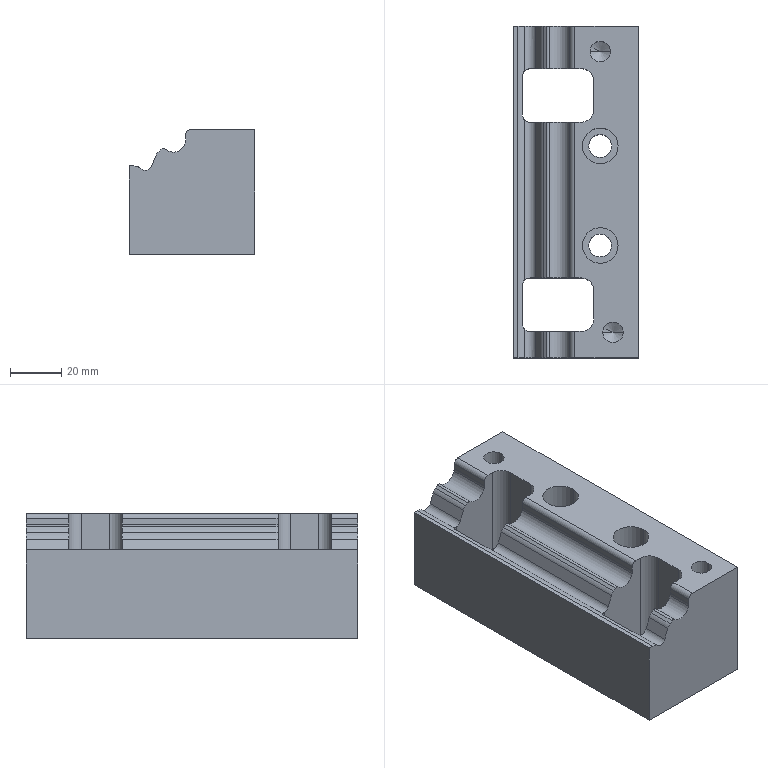Part | 1 solid | 69 faces | box 49 x 130 x 48.948 mm | volume 220865 mm3 | cylinder 39 | plane 26 | cone 4 | commonest cylinder face diameters 9.5 x6 6 x4 8 x4 9 x4 10 x4 14 x4